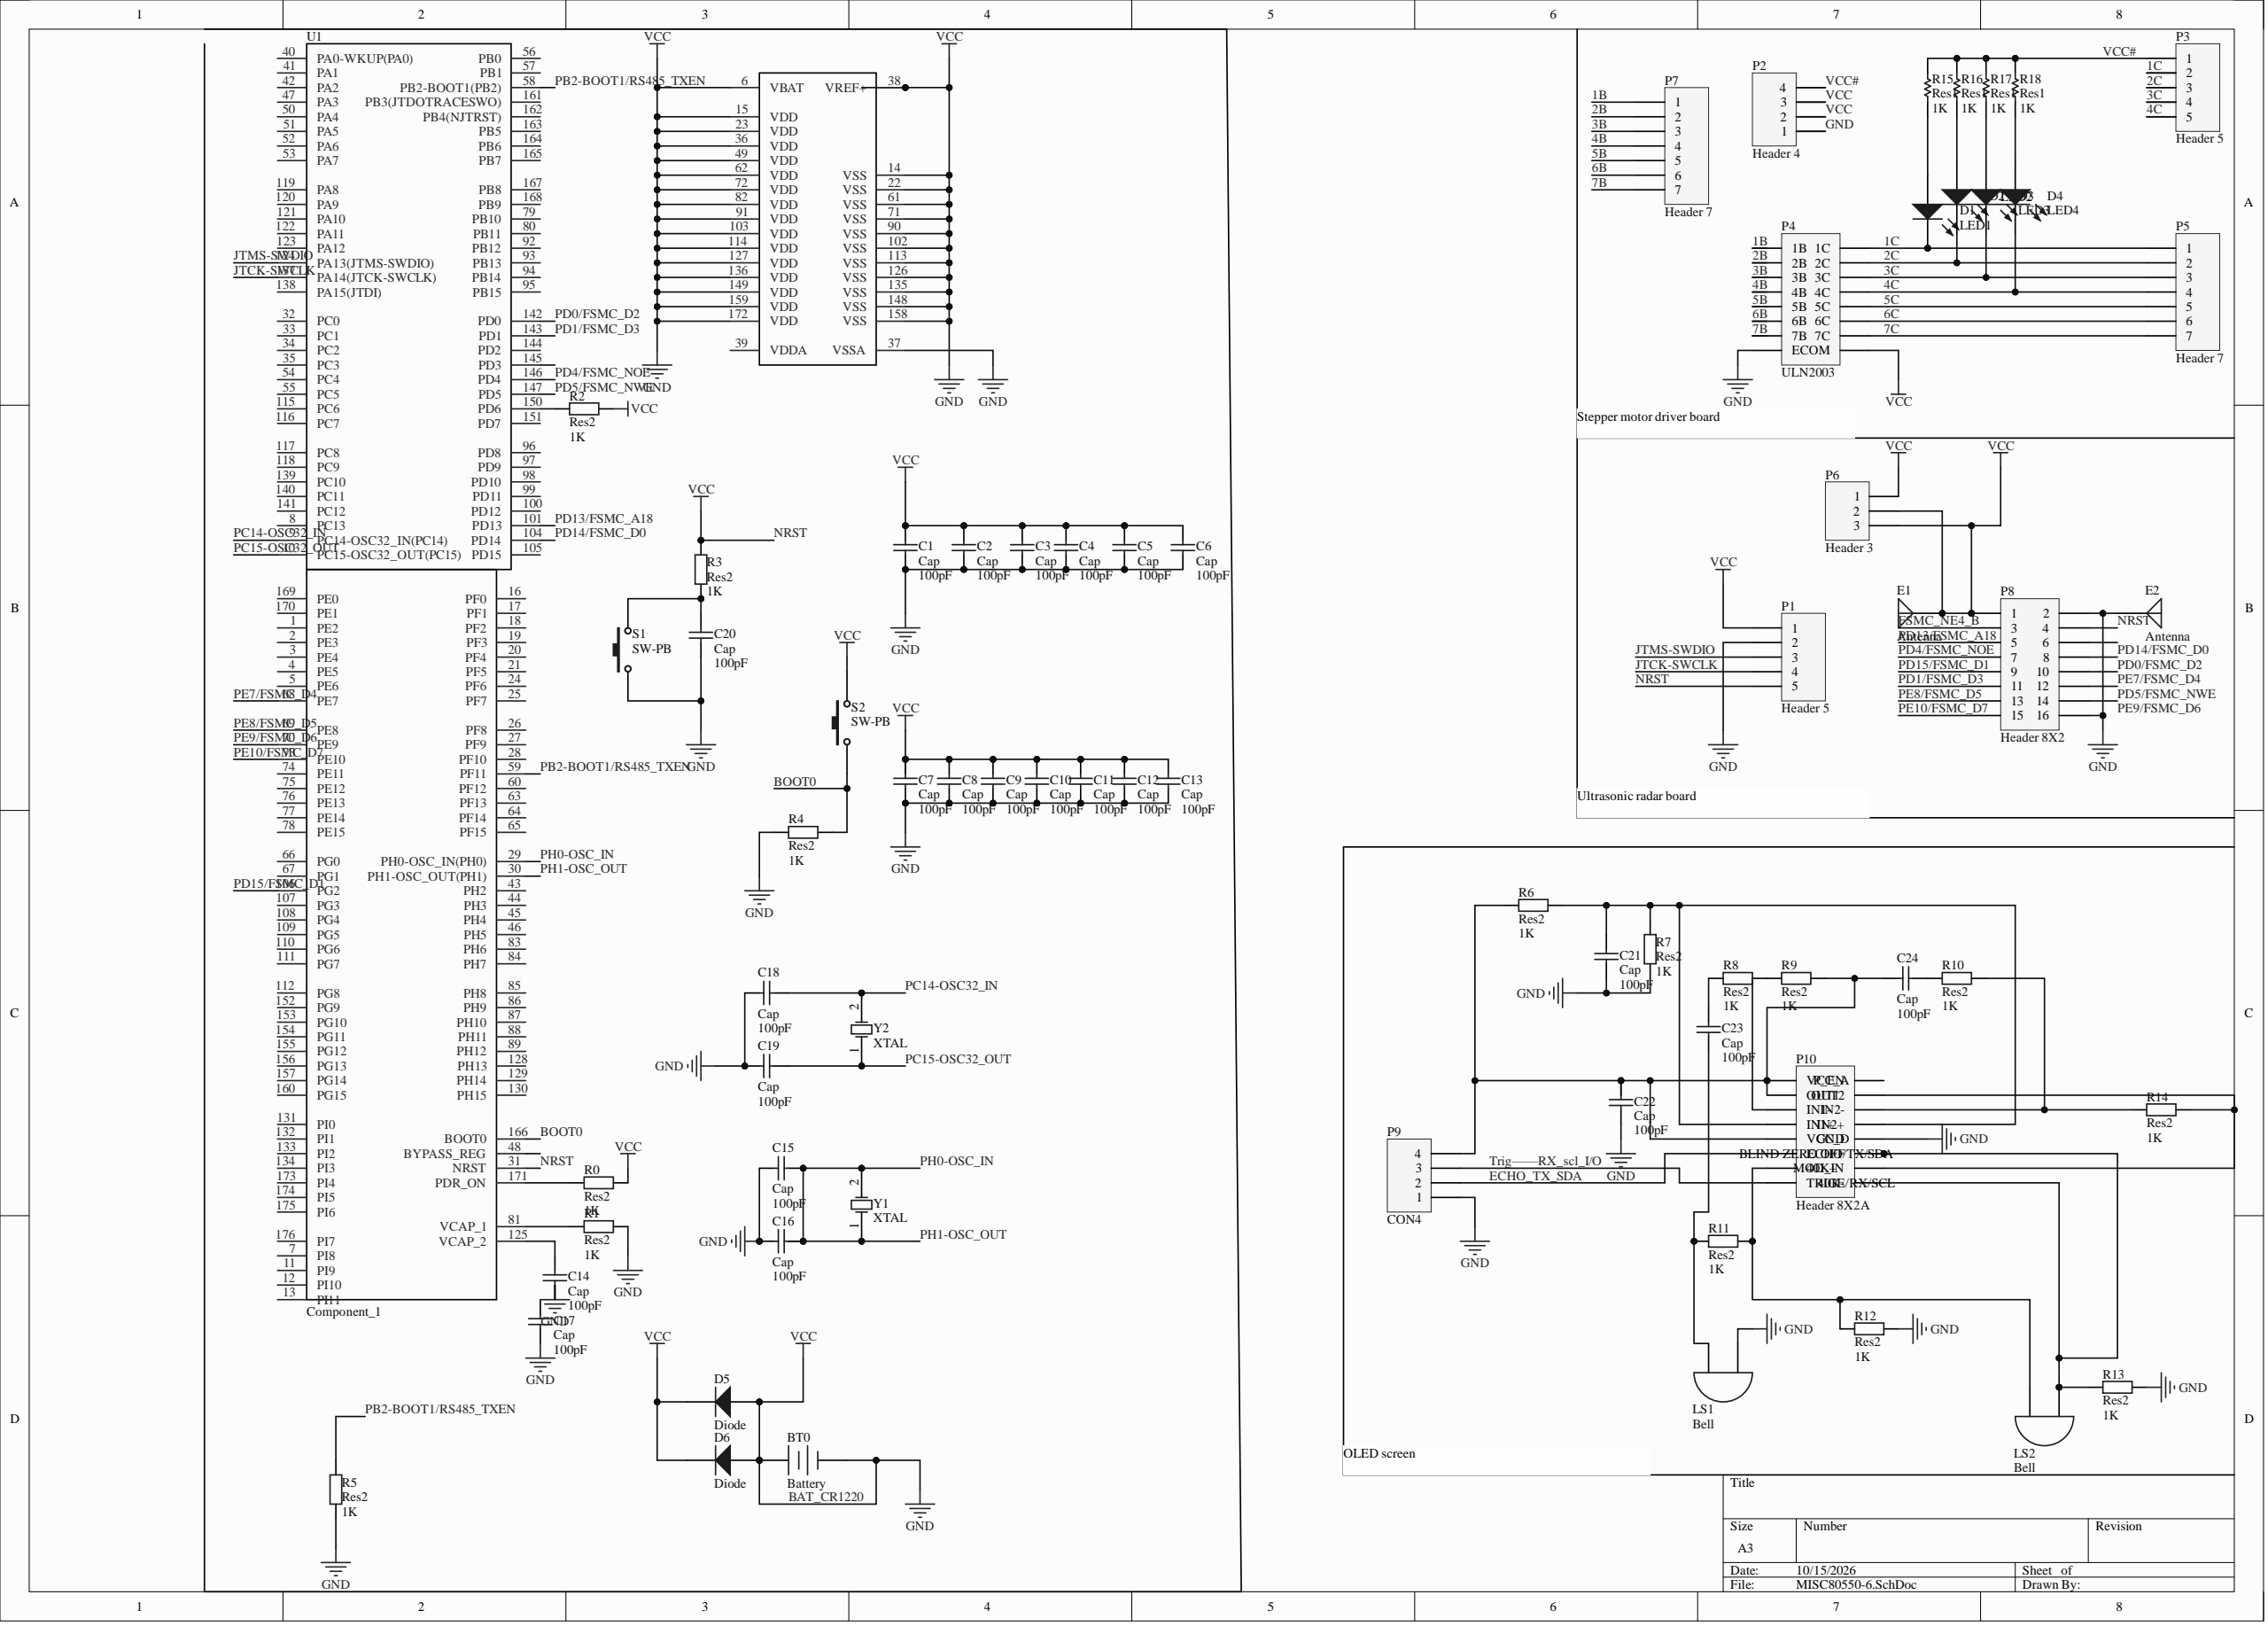Circuit board | Altium Designer | 69 parts | 54 nets
Bill of materials:
Comment,Description,Designator,Footprint,LibRef,Quantity
"Battery","Multicell Battery","BT0","BAT-2","Battery","1"
"Cap","Capacitor","C1, C2, C3, C4, C5, C6, C7, C8, C9, C10, C11, C12, C13, C14, C15, C16, C17, C18, C19, C20, C21, C22, C23, C24","RAD-0.3","Cap","24"
"LED1","Typical INFRARED GaAs LED","D1","LED-0","LED0","1"
"LED2","Typical INFRARED GaAs LED","D2","LED-0","LED0","1"
"LED3","Typical INFRARED GaAs LED","D3","LED-0","LED0","1"
"LED4","Typical INFRARED GaAs LED","D4","LED-0","LED0","1"
"Diode","Default Diode","D5, D6","DSO-C2/X3.3","Diode","2"
"Antenna","Generic Antenna","E1, E2","PIN1","Antenna","2"
"Bell","Electrical Bell","LS1, LS2","PIN2","Bell","2"
"Header 5","Header, 5-Pin","P1, P3","HDR1X5","Header 5","2"
"Header 4","Header, 4-Pin","P2","HDR1X4","Header 4","1"
"ULN2003","ULN2003, Dual row","P4","HDR2X8_CEN","Header 8X2A","1"
"Header 7","Header, 7-Pin","P5, P7","HDR1X7","Header 7","2"
"Header 3","Header, 3-Pin","P6","HDR1X3","Header 3","1"
"Header 8X2","Header, 8-Pin, Dual row","P8","HDR2X8","Header 8X2","1"
"CON4","Header, 4-Pin","P9","HDR1X4","Header 4","1"
"Header 8X2A","Header, 8-Pin, Dual row","P10","HDR2X8_CEN","Header 8X2A","1"
"Res2","Resistor","R0, R1, R2, R3, R4, R5, R6, R7, R8, R9, R10, R11, R12, R13, R14","AXIAL-0.4","Res2","15"
"Res1","Resistor","R15, R16, R17, R18","AXIAL-0.3","Res1","4"
"SW-PB","Switch","S1, S2","SPST-2","SW-PB","2"
"Component_1","","U1","PCBComponent_1","Component_1","1"
"XTAL","Crystal Oscillator","Y1, Y2","BCY-W2/D3.1","XTAL","2"
Netlist (Protel format):
[
BT0
BAT-2
Battery



]
[
C1
RAD-0.3
Cap



]
[
C2
RAD-0.3
Cap



]
[
C3
RAD-0.3
Cap



]
[
C4
RAD-0.3
Cap



]
[
C5
RAD-0.3
Cap



]
[
C6
RAD-0.3
Cap



]
[
C7
RAD-0.3
Cap



]
[
C8
RAD-0.3
Cap



]
[
C9
RAD-0.3
Cap



]
[
C10
RAD-0.3
Cap



]
[
C11
RAD-0.3
Cap



]
[
C12
RAD-0.3
Cap



]
[
C13
RAD-0.3
Cap



]
[
C14
RAD-0.3
Cap



]
[
C15
RAD-0.3
Cap



]
[
C16
RAD-0.3
Cap



]
[
C17
RAD-0.3
Cap



]
[
C18
RAD-0.3
Cap



]
[
C19
RAD-0.3
Cap



]
[
C20
RAD-0.3
Cap



]
[
C21
RAD-0.3
Cap



]
[
C22
RAD-0.3
Cap



]
[
C23
RAD-0.3
Cap



]
[
C24
RAD-0.3
Cap



]
[
D1
LED-0
LED1



]
[
D2
LED-0
LED2



]
[
D3
LED-0
LED3



]
[
D4
LED-0
LED4



]
[
D5
DSO-C2/X3.3
Diode



]
[
D6
DSO-C2/X3.3
Diode



]
[
E1
PIN1
Antenna



]
[
E2
PIN1
Antenna



]
[
LS1
PIN2
Bell



]
[
LS2
PIN2
Bell



]
[
P1
HDR1X5
Header 5



]
[
P2
HDR1X4
Header 4



]
[
P3
HDR1X5
Header 5



]
[
P4
HDR2X8_CEN
ULN2003



]
[
P5
HDR1X7
Header 7



]
[
P6
HDR1X3
Header 3



]
[
P7
HDR1X7
Header 7



]
[
P8
HDR2X8
Header 8X2



]
[
P9
HDR1X4
CON4



]
[
P10
HDR2X8_CEN
Header 8X2A



]
[
R0
AXIAL-0.4
Res2



]
[
R1
AXIAL-0.4
Res2



]
[
R2
AXIAL-0.4
Res2



]
[
R3
AXIAL-0.4
Res2



]
[
R4
AXIAL-0.4
Res2



]
[
R5
AXIAL-0.4
Res2



]
[
R6
AXIAL-0.4
Res2



]
[
R7
AXIAL-0.4
Res2



]
[
R8
AXIAL-0.4
Res2



]
[
R9
AXIAL-0.4
Res2



]
[
R10
AXIAL-0.4
Res2



]
[
R11
AXIAL-0.4
Res2



]
[
R12
AXIAL-0.4
Res2



]
[
R13
AXIAL-0.4
Res2



]
[
R14
AXIAL-0.4
Res2



]
[
R15
AXIAL-0.3
Res1



]
[
R16
AXIAL-0.3
Res1



]
[
R17
AXIAL-0.3
Res1



]
[
R18
AXIAL-0.3
Res1



]
[
S1
SPST-2
SW-PB



]
[
S2
SPST-2
SW-PB



]
[
U1
PCBComponent_1
Component_1



]
[
Y1
BCY-W2/D3.1
XTAL



]
[
Y2
BCY-W2/D3.1
XTAL



]
(
VCC#
P2-4
P3-1
R15-2
R16-2
R17-2
R18-2
)
(
Trig——RX_scl_I/O
P9-3
P10-8
)
(
PH0-OSC_IN
C15-2
C16-2
U1-29
U1-30
Y1-1
Y1-2
)
(
PE10/FSMC_D7
P8-15
U1-73
)
(
PE8/FSMC_D5
P8-13
U1-69
)
(
PE7/FSMC_D4
P8-12
U1-68
)
(
PD15/FSMC_D1
P8-9
U1-106
)
(
PD14/FSMC_D0
P8-8
U1-104
)
(
PD13/FSMC_A18
P8-5
U1-101
)
(
PD5/FSMC_NWE
P8-14
U1-147
)
(
PD4/FSMC_NOE
P8-7
U1-146
)
(
PD1/FSMC_D3
P8-11
U1-143
)
(
PD0/FSMC_D2
P8-10
U1-142
)
(
PC15-OSC32_OUT
C19-2
U1-10
Y2-1
)
(
PC14-OSC32_IN
C18-2
U1-9
Y2-2
)
(
PB2-BOOT1/RS485_TXEN
R5-2
U1-58
U1-59
)
(
NetR8_1
R8-1
R9-2
)
(
NetR2_1
R2-1
U1-150
)
(
NetR1_1
R1-1
U1-81
)
(
NetR0_1
R0-1
U1-171
)
(
NetP10_11
P10-11
R10-1
R14-2
)
(
NetP10_10
P10-10
P10-15
R14-1
)
(
NetLS2_2
LS2-2
P10-7
R11-1
R12-2
)
(
NetLS2_1
LS2-1
P10-14
P10-16
R13-2
)
(
NetD4_1
D4-1
R18-1
)
(
NetD3_1
D3-1
R17-1
)
(
NetD2_1
D2-1
R16-1
)
(
NetD1_1
D1-1
R15-1
)
(
NetC24_1
C24-1
R10-2
)
(
NetC23_2
C23-2
R8-2
)
(
NetC23_1
C23-1
LS1-2
R11-2
)
(
NetC22_2
C22-2
C24-2
P9-4
P10-1
P10-2
P10-5
R6-1
R9-1
)
(
NetC21_2
C21-2
P10-4
P10-12
R6-2
R7-2
)
(
NetC20_2
C20-2
R3-1
S1-2
)
(
NetC14_2
C14-2
U1-125
)
(
JTMS-SWDIO
P1-3
U1-124
)
(
JTCK-SWCLK
P1-4
U1-137
)
(
ECHO_TX_SDA
P9-2
P10-6
)
(
BOOT0
R4-2
S2-1
U1-166
)
(
BAT_CR1220
BT0-1
BT0-2
C1-1
C1-2
C2-1
C2-2
C3-1
C3-2
C4-1
C4-2
C5-1
C5-2
C6-1
C6-2
C7-1
C7-2
C8-1
C8-2
C9-1
C9-2
C10-1
C10-2
C11-1
C11-2
C12-1
C12-2
C13-1
C13-2
C14-1
C15-1
C16-1
C17-1
C18-1
C19-1
C20-1
C21-1
C22-1
D5-1
D5-2
D6-1
D6-2
E1-1
E2-1
LS1-1
P1-1
P1-2
P1-5
P2-1
P2-2
P2-3
P4-8
P4-16
P6-1
P6-2
P6-3
P8-1
P8-2
P8-4
P8-16
P9-1
P10-13
R0-2
R1-2
R2-2
R3-2
R4-1
R5-1
R7-1
R12-1
R13-1
S1-1
S2-2
U1-6
U1-14
U1-15
U1-22
U1-23
U1-31
U1-36
U1-37
U1-38
U1-49
U1-61
U1-62
U1-71
U1-72
U1-82
U1-90
U1-91
U1-102
U1-103
U1-113
U1-114
U1-126
U1-127
U1-135
U1-136
U1-148
U1-149
U1-158
U1-159
U1-172
)
(
7C
P4-15
P5-7
)
(
7B
P4-7
P7-7
)
(
6C
P4-14
P5-6
)
(
6B
P4-6
P7-6
)
(
5C
P4-13
P5-5
)
(
5B
P4-5
P7-5
)
(
4C
D4-2
P3-5
P4-12
P5-4
)
(
4B
P4-4
P7-4
)
(
3C
D3-2
P3-4
P4-11
P5-3
)
(
3B
P4-3
P7-3
)
(
2C
D2-2
P3-3
P4-10
P5-2
)
(
2B
P4-2
P7-2
)
(
1C
D1-2
P3-2
P4-9
P5-1
)
(
1B
P4-1
P7-1
)